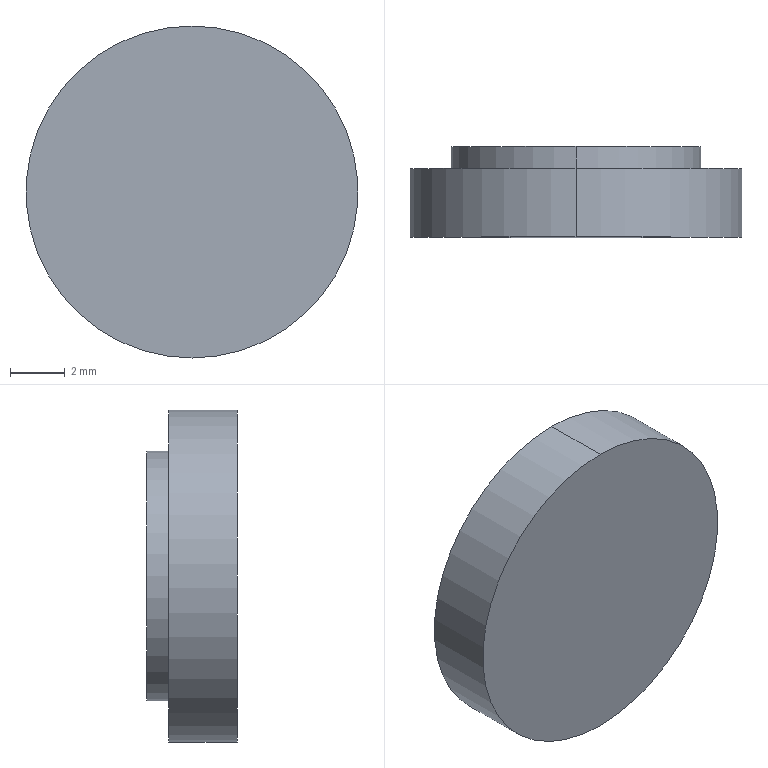Part | STEP file | 4-20.sldasm-Part-165 | 1 solid | 7 faces | box 12.1 x 3.3 x 12.1 mm | volume 339.506 mm3 | cylinder 4 | plane 3 | commonest cylinder face diameters 9.1 x2 12.1 x2
STEP:
#1=CARTESIAN_POINT('',(-190.695,-587.925,-42.55));
#2=VERTEX_POINT('',#1);
#3=CARTESIAN_POINT('',(-190.695,-587.925,-33.45));
#4=VERTEX_POINT('',#3);
#5=CARTESIAN_POINT('',(-190.695,-587.925,-38.));
#6=DIRECTION('',(0.,-1.,0.));
#7=DIRECTION('',(0.,0.,-1.));
#8=AXIS2_PLACEMENT_3D('',#5,#6,#7);
#9=CIRCLE('',#8,4.55);
#10=EDGE_CURVE('',#2,#4,#9,.T.);
#11=ORIENTED_EDGE('',*,*,#10,.F.);
#12=CARTESIAN_POINT('',(-190.695,-587.125,-42.55));
#13=VERTEX_POINT('',#12);
#14=CARTESIAN_POINT('',(-190.695,-587.925,-42.55));
#15=DIRECTION('',(0.,1.,0.));
#16=VECTOR('',#15,1000.);
#17=LINE('',#14,#16);
#18=EDGE_CURVE('',#2,#13,#17,.T.);
#19=ORIENTED_EDGE('',*,*,#18,.T.);
#20=CARTESIAN_POINT('',(-190.695,-587.125,-33.45));
#21=VERTEX_POINT('',#20);
#22=CARTESIAN_POINT('',(-190.695,-587.125,-38.));
#23=DIRECTION('',(0.,-1.,0.));
#24=DIRECTION('',(0.,0.,-1.));
#25=AXIS2_PLACEMENT_3D('',#22,#23,#24);
#26=CIRCLE('',#25,4.55);
#27=EDGE_CURVE('',#13,#21,#26,.T.);
#28=ORIENTED_EDGE('',*,*,#27,.T.);
#29=CARTESIAN_POINT('',(-190.695,-587.925,-33.45));
#30=DIRECTION('',(0.,1.,0.));
#31=VECTOR('',#30,1000.);
#32=LINE('',#29,#31);
#33=EDGE_CURVE('',#4,#21,#32,.T.);
#34=ORIENTED_EDGE('',*,*,#33,.F.);
#35=EDGE_LOOP('',(#11,#19,#28,#34));
#36=FACE_OUTER_BOUND('',#35,.T.);
#37=CARTESIAN_POINT('',(-190.695,-587.925,-38.));
#38=DIRECTION('',(0.,1.,0.));
#39=DIRECTION('',(0.,0.,1.));
#40=AXIS2_PLACEMENT_3D('',#37,#38,#39);
#41=CYLINDRICAL_SURFACE('',#40,4.55);
#42=ADVANCED_FACE('',(#36),#41,.T.);
#43=CARTESIAN_POINT('',(-190.695,-590.425,-44.05));
#44=VERTEX_POINT('',#43);
#45=CARTESIAN_POINT('',(-190.695,-590.425,-31.95));
#46=VERTEX_POINT('',#45);
#47=CARTESIAN_POINT('',(-190.695,-590.425,-38.));
#48=DIRECTION('',(0.,-1.,0.));
#49=DIRECTION('',(0.,0.,-1.));
#50=AXIS2_PLACEMENT_3D('',#47,#48,#49);
#51=CIRCLE('',#50,6.05);
#52=EDGE_CURVE('',#44,#46,#51,.T.);
#53=ORIENTED_EDGE('',*,*,#52,.F.);
#54=CARTESIAN_POINT('',(-190.695,-587.925,-44.05));
#55=VERTEX_POINT('',#54);
#56=CARTESIAN_POINT('',(-190.695,-590.425,-44.05));
#57=DIRECTION('',(0.,1.,0.));
#58=VECTOR('',#57,1000.);
#59=LINE('',#56,#58);
#60=EDGE_CURVE('',#44,#55,#59,.T.);
#61=ORIENTED_EDGE('',*,*,#60,.T.);
#62=CARTESIAN_POINT('',(-190.695,-587.925,-31.95));
#63=VERTEX_POINT('',#62);
#64=CARTESIAN_POINT('',(-190.695,-587.925,-38.));
#65=DIRECTION('',(0.,-1.,0.));
#66=DIRECTION('',(0.,0.,-1.));
#67=AXIS2_PLACEMENT_3D('',#64,#65,#66);
#68=CIRCLE('',#67,6.05);
#69=EDGE_CURVE('',#55,#63,#68,.T.);
#70=ORIENTED_EDGE('',*,*,#69,.T.);
#71=CARTESIAN_POINT('',(-190.695,-590.425,-31.95));
#72=DIRECTION('',(0.,1.,0.));
#73=VECTOR('',#72,1000.);
#74=LINE('',#71,#73);
#75=EDGE_CURVE('',#46,#63,#74,.T.);
#76=ORIENTED_EDGE('',*,*,#75,.F.);
#77=EDGE_LOOP('',(#53,#61,#70,#76));
#78=FACE_OUTER_BOUND('',#77,.T.);
#79=CARTESIAN_POINT('',(-190.695,-590.425,-38.));
#80=DIRECTION('',(0.,1.,0.));
#81=DIRECTION('',(0.,0.,1.));
#82=AXIS2_PLACEMENT_3D('',#79,#80,#81);
#83=CYLINDRICAL_SURFACE('',#82,6.05);
#84=ADVANCED_FACE('',(#78),#83,.T.);
#85=ORIENTED_EDGE('',*,*,#60,.F.);
#86=CARTESIAN_POINT('',(-190.695,-590.425,-38.));
#87=DIRECTION('',(0.,-1.,0.));
#88=DIRECTION('',(0.,0.,-1.));
#89=AXIS2_PLACEMENT_3D('',#86,#87,#88);
#90=CIRCLE('',#89,6.05);
#91=EDGE_CURVE('',#46,#44,#90,.T.);
#92=ORIENTED_EDGE('',*,*,#91,.F.);
#93=ORIENTED_EDGE('',*,*,#75,.T.);
#94=CARTESIAN_POINT('',(-190.695,-587.925,-38.));
#95=DIRECTION('',(0.,-1.,0.));
#96=DIRECTION('',(0.,0.,-1.));
#97=AXIS2_PLACEMENT_3D('',#94,#95,#96);
#98=CIRCLE('',#97,6.05);
#99=EDGE_CURVE('',#63,#55,#98,.T.);
#100=ORIENTED_EDGE('',*,*,#99,.T.);
#101=EDGE_LOOP('',(#85,#92,#93,#100));
#102=FACE_OUTER_BOUND('',#101,.T.);
#103=CARTESIAN_POINT('',(-190.695,-590.425,-38.));
#104=DIRECTION('',(0.,1.,0.));
#105=DIRECTION('',(0.,0.,1.));
#106=AXIS2_PLACEMENT_3D('',#103,#104,#105);
#107=CYLINDRICAL_SURFACE('',#106,6.05);
#108=ADVANCED_FACE('',(#102),#107,.T.);
#109=ORIENTED_EDGE('',*,*,#91,.T.);
#110=ORIENTED_EDGE('',*,*,#52,.T.);
#111=EDGE_LOOP('',(#109,#110));
#112=FACE_OUTER_BOUND('',#111,.T.);
#113=CARTESIAN_POINT('',(-190.695,-590.425,-38.));
#114=DIRECTION('',(0.,-1.,0.));
#115=DIRECTION('',(0.,0.,-1.));
#116=AXIS2_PLACEMENT_3D('',#113,#114,#115);
#117=PLANE('',#116);
#118=ADVANCED_FACE('',(#112),#117,.T.);
#119=CARTESIAN_POINT('',(-190.695,-587.925,-38.));
#120=DIRECTION('',(0.,-1.,0.));
#121=DIRECTION('',(0.,0.,-1.));
#122=AXIS2_PLACEMENT_3D('',#119,#120,#121);
#123=CIRCLE('',#122,4.55);
#124=EDGE_CURVE('',#4,#2,#123,.T.);
#125=ORIENTED_EDGE('',*,*,#124,.T.);
#126=ORIENTED_EDGE('',*,*,#10,.T.);
#127=EDGE_LOOP('',(#125,#126));
#128=FACE_BOUND('',#127,.T.);
#129=ORIENTED_EDGE('',*,*,#99,.F.);
#130=ORIENTED_EDGE('',*,*,#69,.F.);
#131=EDGE_LOOP('',(#129,#130));
#132=FACE_OUTER_BOUND('',#131,.T.);
#133=CARTESIAN_POINT('',(-190.695,-587.925,-38.));
#134=DIRECTION('',(0.,-1.,0.));
#135=DIRECTION('',(0.,0.,-1.));
#136=AXIS2_PLACEMENT_3D('',#133,#134,#135);
#137=PLANE('',#136);
#138=ADVANCED_FACE('',(#128,#132),#137,.F.);
#139=ORIENTED_EDGE('',*,*,#18,.F.);
#140=ORIENTED_EDGE('',*,*,#124,.F.);
#141=ORIENTED_EDGE('',*,*,#33,.T.);
#142=CARTESIAN_POINT('',(-190.695,-587.125,-38.));
#143=DIRECTION('',(0.,-1.,0.));
#144=DIRECTION('',(0.,0.,-1.));
#145=AXIS2_PLACEMENT_3D('',#142,#143,#144);
#146=CIRCLE('',#145,4.55);
#147=EDGE_CURVE('',#21,#13,#146,.T.);
#148=ORIENTED_EDGE('',*,*,#147,.T.);
#149=EDGE_LOOP('',(#139,#140,#141,#148));
#150=FACE_OUTER_BOUND('',#149,.T.);
#151=CARTESIAN_POINT('',(-190.695,-587.925,-38.));
#152=DIRECTION('',(0.,1.,0.));
#153=DIRECTION('',(0.,0.,1.));
#154=AXIS2_PLACEMENT_3D('',#151,#152,#153);
#155=CYLINDRICAL_SURFACE('',#154,4.55);
#156=ADVANCED_FACE('',(#150),#155,.T.);
#157=ORIENTED_EDGE('',*,*,#147,.F.);
#158=ORIENTED_EDGE('',*,*,#27,.F.);
#159=EDGE_LOOP('',(#157,#158));
#160=FACE_OUTER_BOUND('',#159,.T.);
#161=CARTESIAN_POINT('',(-190.695,-587.125,-38.));
#162=DIRECTION('',(0.,-1.,0.));
#163=DIRECTION('',(0.,0.,-1.));
#164=AXIS2_PLACEMENT_3D('',#161,#162,#163);
#165=PLANE('',#164);
#166=ADVANCED_FACE('',(#160),#165,.F.);
#167=CLOSED_SHELL('',(#42,#84,#108,#118,#138,#156,#166));
#168=MANIFOLD_SOLID_BREP('',#167);
#169=CARTESIAN_POINT('',(0.,0.,0.));
#170=DIRECTION('',(0.,0.,1.));
#171=DIRECTION('',(1.,0.,0.));
#172=AXIS2_PLACEMENT_3D('',#169,#170,#171);
#173=(LENGTH_UNIT()NAMED_UNIT(*)SI_UNIT(.MILLI.,.METRE.));
#174=UNCERTAINTY_MEASURE_WITH_UNIT(LENGTH_MEASURE(0.00001),#173,'','');
#175=(NAMED_UNIT(*)PLANE_ANGLE_UNIT()SI_UNIT($,.RADIAN.));
#176=(NAMED_UNIT(*)SI_UNIT($,.STERADIAN.)SOLID_ANGLE_UNIT());
#177=(GEOMETRIC_REPRESENTATION_CONTEXT(3)GLOBAL_UNCERTAINTY_ASSIGNED_CONTEXT((#174))GLOBAL_UNIT_ASSIGNED_CONTEXT((#173,#175,#176))REPRESENTATION_CONTEXT('',''));
#178=ADVANCED_BREP_SHAPE_REPRESENTATION('',(#168,#172),#177);